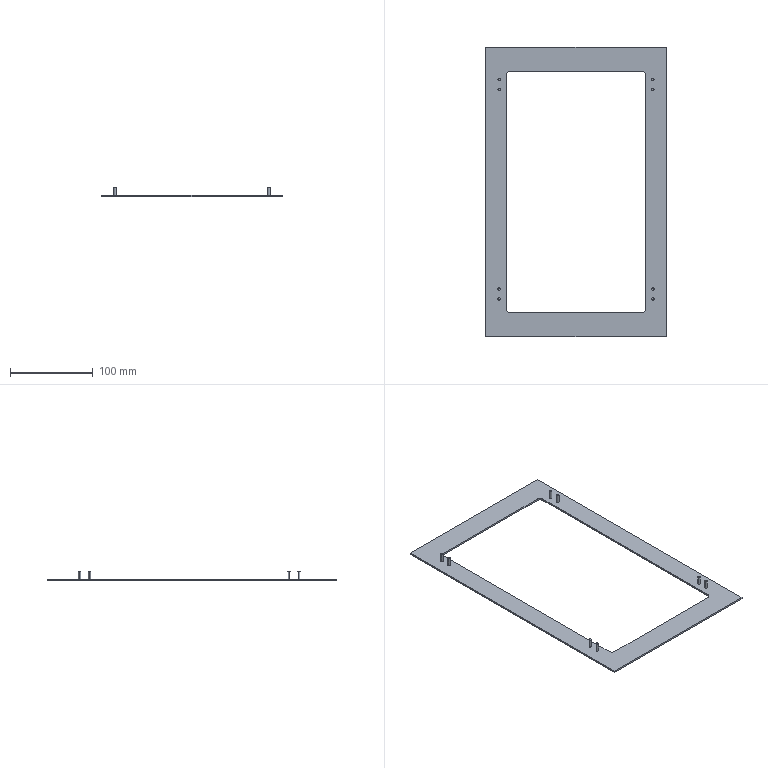Part | SolidWorks | features ICE 3, Fillet 1, FlatPattern 1, SMBaseFlange 1, SheetMetal 1 | 9 solids | 62 faces | box 218 x 350 x 12 mm | volume 54399 mm3 | cylinder 36 | plane 26 | commonest cylinder face diameters 3 x32 10 x4